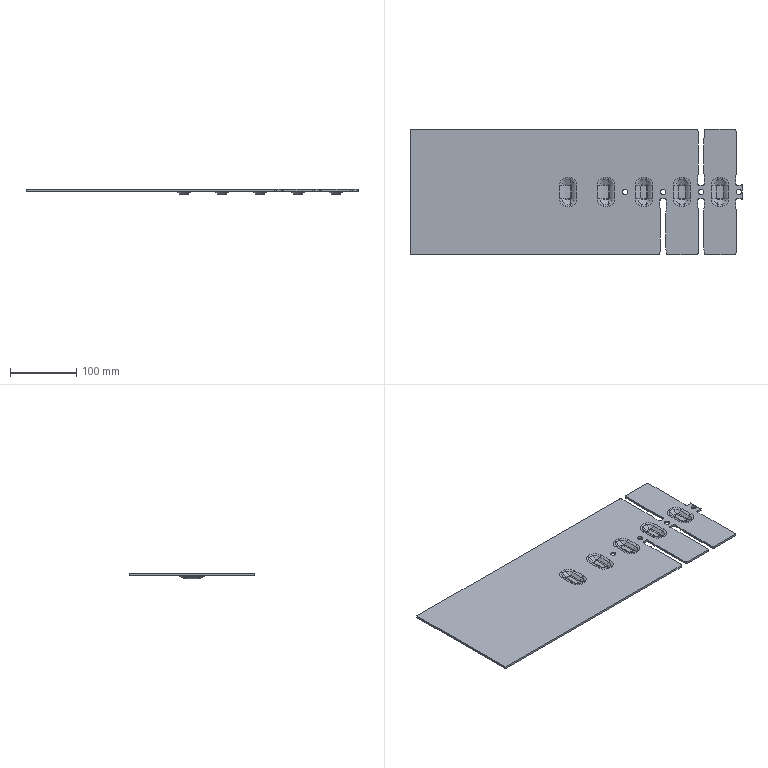Part | STEP file | 1_id298_x_t | 1 solid | 322 faces | box 499.877 x 188.495 x 8.554 mm | volume 279674 mm3 | spline 180 | cylinder 85 | plane 53 | other 4 | commonest cylinder face diameters 6 x28 12.15 x20 3 x18 101.133 x8 2205 x7 8.06 x4